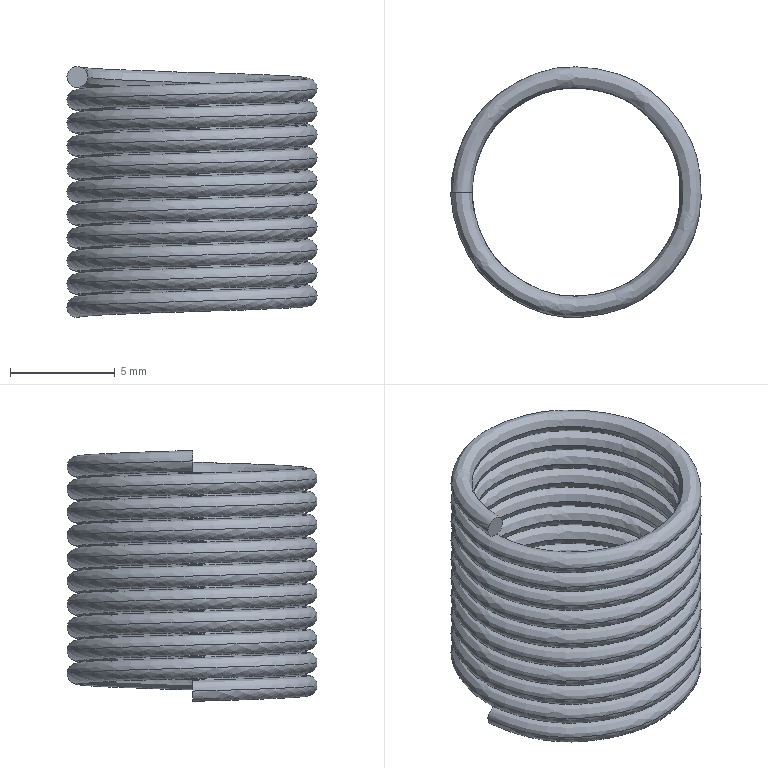Part | SolidWorks | features BaseBody 1 | 1 solid | 4 faces | box 11.964 x 11.962 x 11.998 mm | volume 268.537 mm3 | spline 2 | plane 2